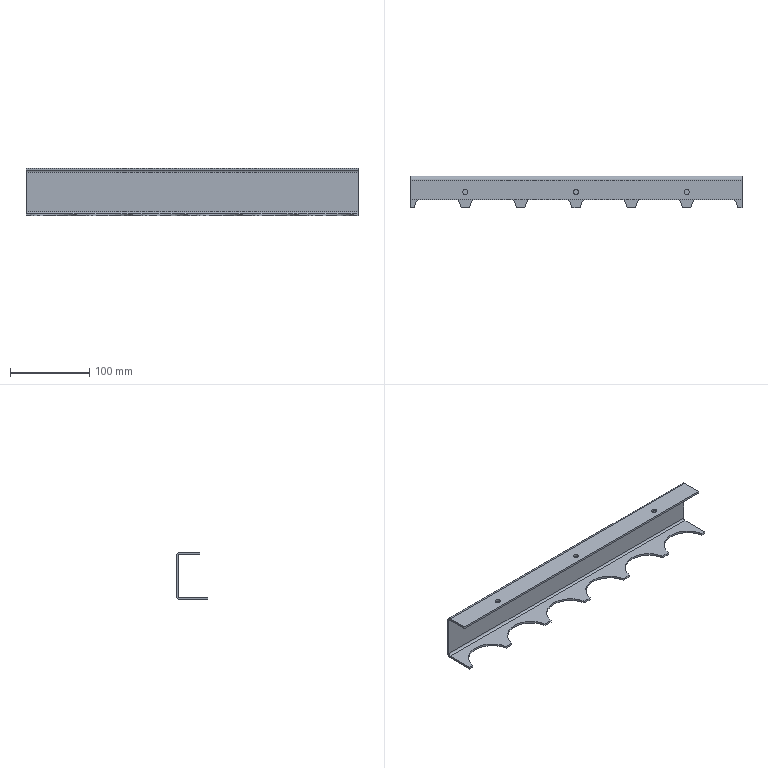Part | STEP file | cc-coverrollers-05 | 1 solid | 29 faces | box 418.8 x 40 x 60 mm | volume 110529 mm3 | plane 16 | cylinder 10 | spline 3 | commonest cylinder face diameters 60 x6 5 x2 10 x2